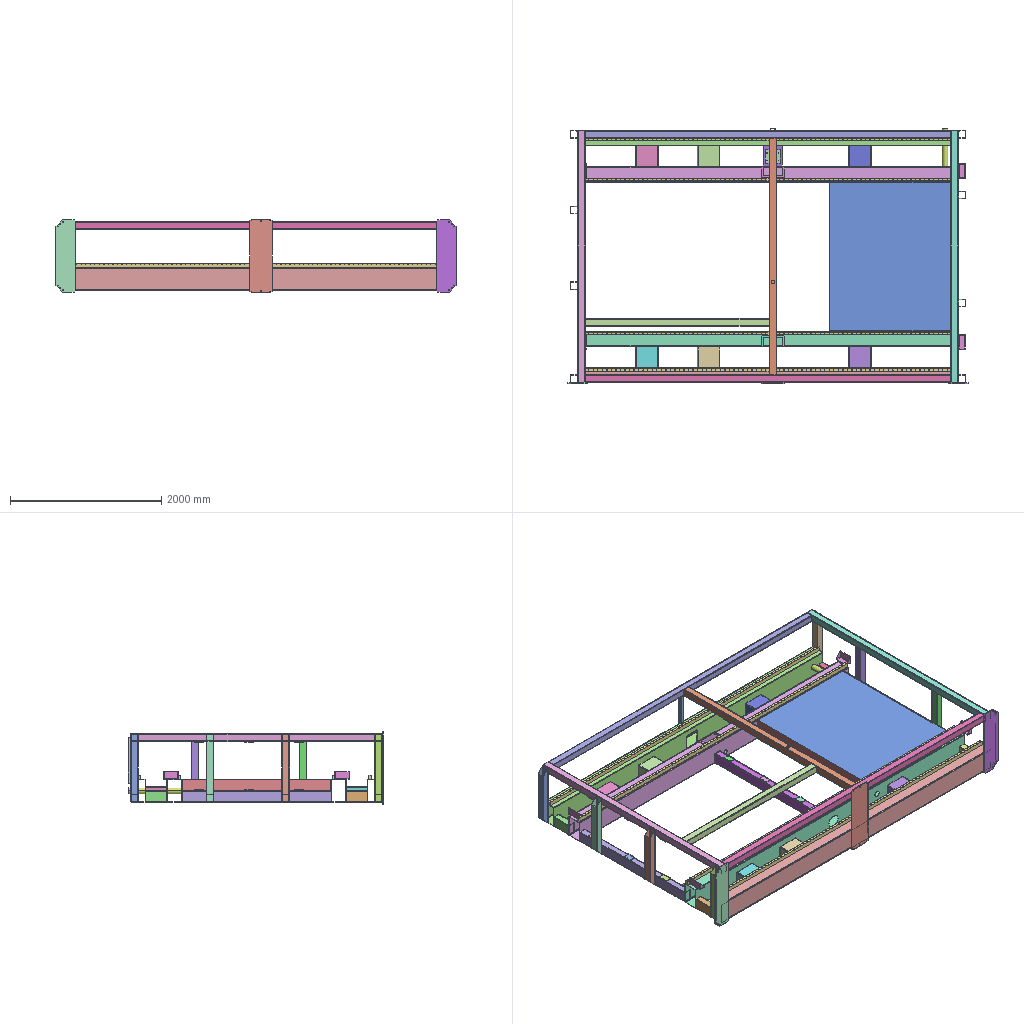Assembly | SolidWorks | 8 different items | 15 placed | box 5290 x 3374 x 970 mm
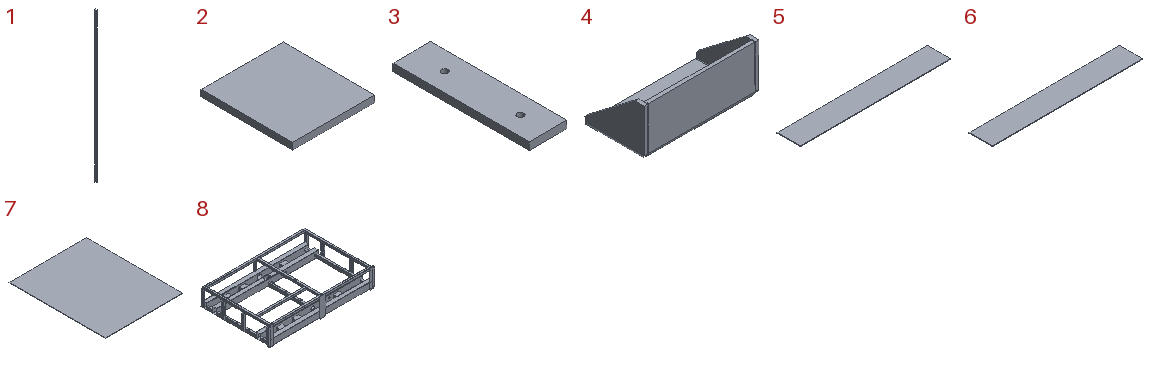Parts list (item | quantity | size | volume | features):
1 | x4 | 30 x 55 x 5030 mm | 8266814 mm3 | features BaseBody 1
2 | x1 | 250 x 280 x 20 mm | 1400000 mm3 | features BaseBody 1
3 | x2 | 50 x 180 x 10 mm | 88865 mm3 | features BaseBody 1, ICE 1
4 | x4 | 194 x 100 x 80 mm | 247792 mm3 | features Chamfer 2, CornerFeat 2, EdgeFlange 2, FlatPattern 1, SMBaseFlange 1, SheetMetal 1
5 | x1 | 1968 x 300 x 8 mm | 4723200 mm3 | features BaseBody 1, MoveFace 1
6 | x1 | 1968 x 300 x 8 mm | 4723200 mm3 | features BaseBody 1, MoveFace 1
7 | x1 | 1590 x 1968 x 8 mm | 25032960 mm3 | features BaseBody 1, MoveFace 1
8 | x1 | 5290 x 3374 x 970 mm | 176959507 mm3 | features BaseBody 30, ICE 19, Chamfer 2, EdgeFlange 1, FlatPattern 1, LPattern 1, MirrorSolid 1, MoveFace 1, SMBaseFlange 1, SheetMetal 1
Mates (type | each side: item.copy, entity, surface, feature):
Width | 3.1 face plane Input 1 | 3.1 face plane Input 1 | 8.1 face plane Input 29 | 8.1 face plane Input 28
Coincident | 2.1 face plane Input 1 | 3.1 face plane Input 1
Coincident | 3.1 face plane Input 1 | 3.2 face plane Input 1
Coincident | 2.1 face plane Input 1 | 3.2 face plane Input 1
Width | 3.2 face plane Input 1 | 3.1 face plane Input 1 | 2.1 face plane Input 1 | 2.1 face plane Input 1
DistanceDim | 3.1 face cylinder Cut-Extrude1 | 3.2 face cylinder Cut-Extrude1
Coincident | 5.1 face plane Input 1 | 6.1 face plane Input 1 | 2 times
Coincident | 7.1 face plane Input 1 | 6.1 face plane Input 1 | 3 times
Coincident | 5.1 face plane Input 1 | 7.1 face plane Input 1
Coincident | 8.1 face plane Input 12 | 6.1 face plane Input 1 | 2 times
Coincident | 8.1 face plane Input 29 | 6.1 face plane Input 1
Coincident | 8.1 face plane Input 29 | 4.1 face plane Base-Flange1
Parallel | 8.1 face plane Input 29 | 4.1 face plane Edge-Flange2
Coincident | 1.1 face plane Input 1 | 4.1 face plane Edge-Flange2
Coincident | 1.2 face plane Input 1 | 4.2 face plane Edge-Flange2
Coincident | 8.1 face plane Input 30 | 4.2 face plane Base-Flange1